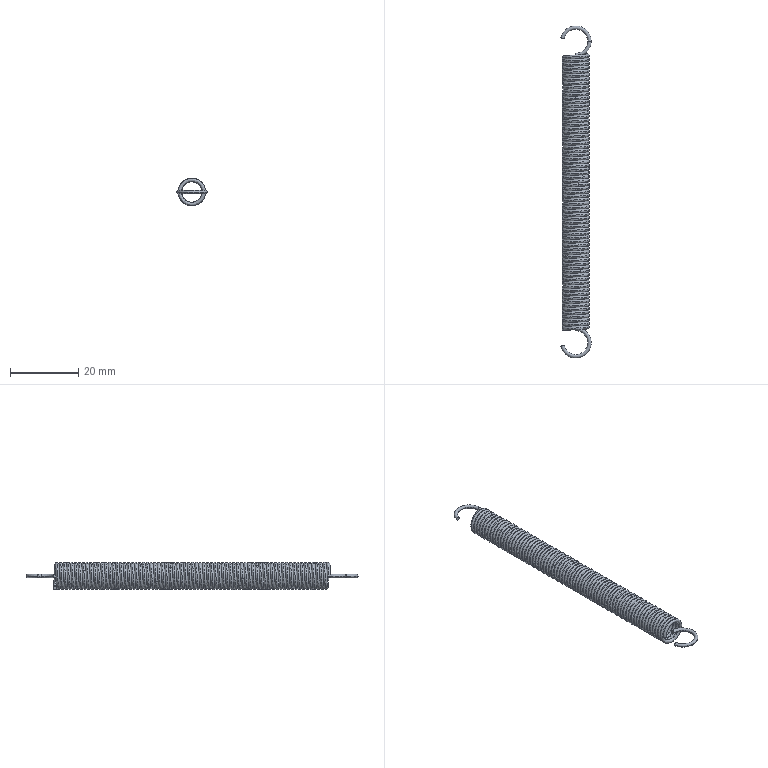Part | SolidWorks | features BaseBody 3, ICE 1, RefAxis 1 | 3 solids | 50 faces | box 8.882 x 97 x 8 mm | volume 1277 mm3 | spline 38 | torus 6 | plane 6